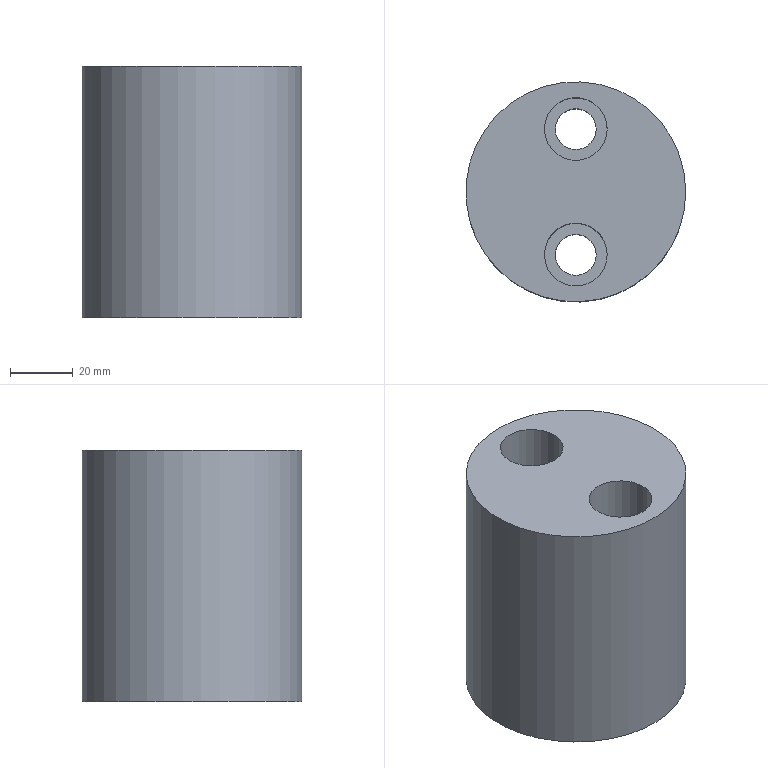Part | NX | features solid 2 | 1 solid | 9 faces | box 70 x 70 x 80 mm | volume 268496 mm3 | cylinder 5 | plane 4 | commonest cylinder face diameters 13 x2 20 x2 70 x1
STEP:
#1=CARTESIAN_POINT('',(-354.,100.,125.));
#2=VERTEX_POINT('',#1);
#3=CARTESIAN_POINT('',(-389.,100.,125.));
#4=DIRECTION('',(0.,0.,1.));
#5=DIRECTION('',(1.,0.,0.));
#6=AXIS2_PLACEMENT_3D('',#3,#4,#5);
#7=CIRCLE('',#6,35.);
#8=EDGE_CURVE('',#2,#2,#7,.T.);
#9=ORIENTED_EDGE('',*,*,#8,.T.);
#10=EDGE_LOOP('',(#9));
#11=FACE_BOUND('',#10,.T.);
#12=CARTESIAN_POINT('',(-354.,100.,205.));
#13=VERTEX_POINT('',#12);
#14=CARTESIAN_POINT('',(-389.,100.,205.));
#15=DIRECTION('',(0.,0.,1.));
#16=DIRECTION('',(1.,0.,0.));
#17=AXIS2_PLACEMENT_3D('',#14,#15,#16);
#18=CIRCLE('',#17,35.);
#19=EDGE_CURVE('',#13,#13,#18,.T.);
#20=ORIENTED_EDGE('',*,*,#19,.F.);
#21=EDGE_LOOP('',(#20));
#22=FACE_BOUND('',#21,.T.);
#23=CARTESIAN_POINT('',(-389.,100.,-95.));
#24=DIRECTION('',(0.,0.,1.));
#25=DIRECTION('',(1.,0.,0.));
#26=AXIS2_PLACEMENT_3D('',#23,#24,#25);
#27=CYLINDRICAL_SURFACE('',#26,35.);
#28=ADVANCED_FACE('',(#11,#22),#27,.T.);
#29=CARTESIAN_POINT('',(-382.5,120.,125.));
#30=VERTEX_POINT('',#29);
#31=CARTESIAN_POINT('',(-389.,120.,125.));
#32=DIRECTION('',(0.,0.,1.));
#33=DIRECTION('',(1.,0.,0.));
#34=AXIS2_PLACEMENT_3D('',#31,#32,#33);
#35=CIRCLE('',#34,6.5);
#36=EDGE_CURVE('',#30,#30,#35,.T.);
#37=ORIENTED_EDGE('',*,*,#36,.T.);
#38=EDGE_LOOP('',(#37));
#39=FACE_BOUND('',#38,.T.);
#40=CARTESIAN_POINT('',(-382.5,80.,125.));
#41=VERTEX_POINT('',#40);
#42=CARTESIAN_POINT('',(-389.,80.,125.));
#43=DIRECTION('',(0.,0.,1.));
#44=DIRECTION('',(1.,0.,0.));
#45=AXIS2_PLACEMENT_3D('',#42,#43,#44);
#46=CIRCLE('',#45,6.5);
#47=EDGE_CURVE('',#41,#41,#46,.T.);
#48=ORIENTED_EDGE('',*,*,#47,.T.);
#49=EDGE_LOOP('',(#48));
#50=FACE_BOUND('',#49,.T.);
#51=ORIENTED_EDGE('',*,*,#8,.F.);
#52=EDGE_LOOP('',(#51));
#53=FACE_BOUND('',#52,.T.);
#54=CARTESIAN_POINT('',(-389.,100.,125.));
#55=DIRECTION('',(0.,0.,1.));
#56=DIRECTION('',(1.,0.,0.));
#57=AXIS2_PLACEMENT_3D('',#54,#55,#56);
#58=PLANE('',#57);
#59=ADVANCED_FACE('',(#39,#50,#53),#58,.F.);
#60=CARTESIAN_POINT('',(-379.,120.,205.));
#61=VERTEX_POINT('',#60);
#62=CARTESIAN_POINT('',(-389.,120.,205.));
#63=DIRECTION('',(0.,0.,1.));
#64=DIRECTION('',(1.,0.,0.));
#65=AXIS2_PLACEMENT_3D('',#62,#63,#64);
#66=CIRCLE('',#65,10.);
#67=EDGE_CURVE('',#61,#61,#66,.T.);
#68=ORIENTED_EDGE('',*,*,#67,.F.);
#69=EDGE_LOOP('',(#68));
#70=FACE_BOUND('',#69,.T.);
#71=CARTESIAN_POINT('',(-379.,80.,205.));
#72=VERTEX_POINT('',#71);
#73=CARTESIAN_POINT('',(-389.,80.,205.));
#74=DIRECTION('',(0.,0.,1.));
#75=DIRECTION('',(1.,0.,0.));
#76=AXIS2_PLACEMENT_3D('',#73,#74,#75);
#77=CIRCLE('',#76,10.);
#78=EDGE_CURVE('',#72,#72,#77,.T.);
#79=ORIENTED_EDGE('',*,*,#78,.F.);
#80=EDGE_LOOP('',(#79));
#81=FACE_BOUND('',#80,.T.);
#82=ORIENTED_EDGE('',*,*,#19,.T.);
#83=EDGE_LOOP('',(#82));
#84=FACE_BOUND('',#83,.T.);
#85=CARTESIAN_POINT('',(-389.,100.,205.));
#86=DIRECTION('',(0.,0.,1.));
#87=DIRECTION('',(1.,0.,0.));
#88=AXIS2_PLACEMENT_3D('',#85,#86,#87);
#89=PLANE('',#88);
#90=ADVANCED_FACE('',(#70,#81,#84),#89,.T.);
#91=CARTESIAN_POINT('',(-395.5,80.,155.));
#92=VERTEX_POINT('',#91);
#93=CARTESIAN_POINT('',(-389.,80.,155.));
#94=DIRECTION('',(0.,0.,-1.));
#95=DIRECTION('',(-1.,0.,0.));
#96=AXIS2_PLACEMENT_3D('',#93,#94,#95);
#97=CIRCLE('',#96,6.5);
#98=EDGE_CURVE('',#92,#92,#97,.F.);
#99=ORIENTED_EDGE('',*,*,#98,.T.);
#100=EDGE_LOOP('',(#99));
#101=FACE_BOUND('',#100,.T.);
#102=ORIENTED_EDGE('',*,*,#47,.F.);
#103=EDGE_LOOP('',(#102));
#104=FACE_BOUND('',#103,.T.);
#105=CARTESIAN_POINT('',(-389.,80.,95.));
#106=DIRECTION('',(0.,0.,1.));
#107=DIRECTION('',(1.,0.,0.));
#108=AXIS2_PLACEMENT_3D('',#105,#106,#107);
#109=CYLINDRICAL_SURFACE('',#108,6.5);
#110=ADVANCED_FACE('',(#101,#104),#109,.F.);
#111=ORIENTED_EDGE('',*,*,#98,.F.);
#112=EDGE_LOOP('',(#111));
#113=FACE_BOUND('',#112,.T.);
#114=CARTESIAN_POINT('',(-379.,80.,155.));
#115=VERTEX_POINT('',#114);
#116=CARTESIAN_POINT('',(-389.,80.,155.));
#117=DIRECTION('',(0.,0.,1.));
#118=DIRECTION('',(1.,0.,0.));
#119=AXIS2_PLACEMENT_3D('',#116,#117,#118);
#120=CIRCLE('',#119,10.);
#121=EDGE_CURVE('',#115,#115,#120,.T.);
#122=ORIENTED_EDGE('',*,*,#121,.T.);
#123=EDGE_LOOP('',(#122));
#124=FACE_BOUND('',#123,.T.);
#125=CARTESIAN_POINT('',(-389.,80.,155.));
#126=DIRECTION('',(0.,0.,-1.));
#127=DIRECTION('',(-1.,0.,0.));
#128=AXIS2_PLACEMENT_3D('',#125,#126,#127);
#129=PLANE('',#128);
#130=ADVANCED_FACE('',(#113,#124),#129,.F.);
#131=ORIENTED_EDGE('',*,*,#78,.T.);
#132=EDGE_LOOP('',(#131));
#133=FACE_BOUND('',#132,.T.);
#134=ORIENTED_EDGE('',*,*,#121,.F.);
#135=EDGE_LOOP('',(#134));
#136=FACE_BOUND('',#135,.T.);
#137=CARTESIAN_POINT('',(-389.,80.,155.));
#138=DIRECTION('',(0.,0.,1.));
#139=DIRECTION('',(1.,0.,0.));
#140=AXIS2_PLACEMENT_3D('',#137,#138,#139);
#141=CYLINDRICAL_SURFACE('',#140,10.);
#142=ADVANCED_FACE('',(#133,#136),#141,.F.);
#143=CARTESIAN_POINT('',(-395.5,120.,155.));
#144=VERTEX_POINT('',#143);
#145=CARTESIAN_POINT('',(-389.,120.,155.));
#146=DIRECTION('',(0.,0.,-1.));
#147=DIRECTION('',(-1.,0.,0.));
#148=AXIS2_PLACEMENT_3D('',#145,#146,#147);
#149=CIRCLE('',#148,6.5);
#150=EDGE_CURVE('',#144,#144,#149,.F.);
#151=ORIENTED_EDGE('',*,*,#150,.T.);
#152=EDGE_LOOP('',(#151));
#153=FACE_BOUND('',#152,.T.);
#154=ORIENTED_EDGE('',*,*,#36,.F.);
#155=EDGE_LOOP('',(#154));
#156=FACE_BOUND('',#155,.T.);
#157=CARTESIAN_POINT('',(-389.,120.,95.));
#158=DIRECTION('',(0.,0.,1.));
#159=DIRECTION('',(1.,0.,0.));
#160=AXIS2_PLACEMENT_3D('',#157,#158,#159);
#161=CYLINDRICAL_SURFACE('',#160,6.5);
#162=ADVANCED_FACE('',(#153,#156),#161,.F.);
#163=ORIENTED_EDGE('',*,*,#150,.F.);
#164=EDGE_LOOP('',(#163));
#165=FACE_BOUND('',#164,.T.);
#166=CARTESIAN_POINT('',(-379.,120.,155.));
#167=VERTEX_POINT('',#166);
#168=CARTESIAN_POINT('',(-389.,120.,155.));
#169=DIRECTION('',(0.,0.,1.));
#170=DIRECTION('',(1.,0.,0.));
#171=AXIS2_PLACEMENT_3D('',#168,#169,#170);
#172=CIRCLE('',#171,10.);
#173=EDGE_CURVE('',#167,#167,#172,.T.);
#174=ORIENTED_EDGE('',*,*,#173,.T.);
#175=EDGE_LOOP('',(#174));
#176=FACE_BOUND('',#175,.T.);
#177=CARTESIAN_POINT('',(-389.,120.,155.));
#178=DIRECTION('',(0.,0.,-1.));
#179=DIRECTION('',(-1.,0.,0.));
#180=AXIS2_PLACEMENT_3D('',#177,#178,#179);
#181=PLANE('',#180);
#182=ADVANCED_FACE('',(#165,#176),#181,.F.);
#183=ORIENTED_EDGE('',*,*,#67,.T.);
#184=EDGE_LOOP('',(#183));
#185=FACE_BOUND('',#184,.T.);
#186=ORIENTED_EDGE('',*,*,#173,.F.);
#187=EDGE_LOOP('',(#186));
#188=FACE_BOUND('',#187,.T.);
#189=CARTESIAN_POINT('',(-389.,120.,155.));
#190=DIRECTION('',(0.,0.,1.));
#191=DIRECTION('',(1.,0.,0.));
#192=AXIS2_PLACEMENT_3D('',#189,#190,#191);
#193=CYLINDRICAL_SURFACE('',#192,10.);
#194=ADVANCED_FACE('',(#185,#188),#193,.F.);
#195=CLOSED_SHELL('',(#28,#59,#90,#110,#130,#142,#162,#182,#194));
#196=MANIFOLD_SOLID_BREP('',#195);
#197=(LENGTH_UNIT()NAMED_UNIT(*)SI_UNIT(.MILLI.,.METRE.));
#198=UNCERTAINTY_MEASURE_WITH_UNIT(LENGTH_MEASURE(0.00001),#197,'','');
#199=(NAMED_UNIT(*)PLANE_ANGLE_UNIT()SI_UNIT($,.RADIAN.));
#200=(NAMED_UNIT(*)SI_UNIT($,.STERADIAN.)SOLID_ANGLE_UNIT());
#201=(GEOMETRIC_REPRESENTATION_CONTEXT(3)GLOBAL_UNCERTAINTY_ASSIGNED_CONTEXT((#198))GLOBAL_UNIT_ASSIGNED_CONTEXT((#197,#199,#200))REPRESENTATION_CONTEXT('',''));
#202=ADVANCED_BREP_SHAPE_REPRESENTATION('',(#196),#201);